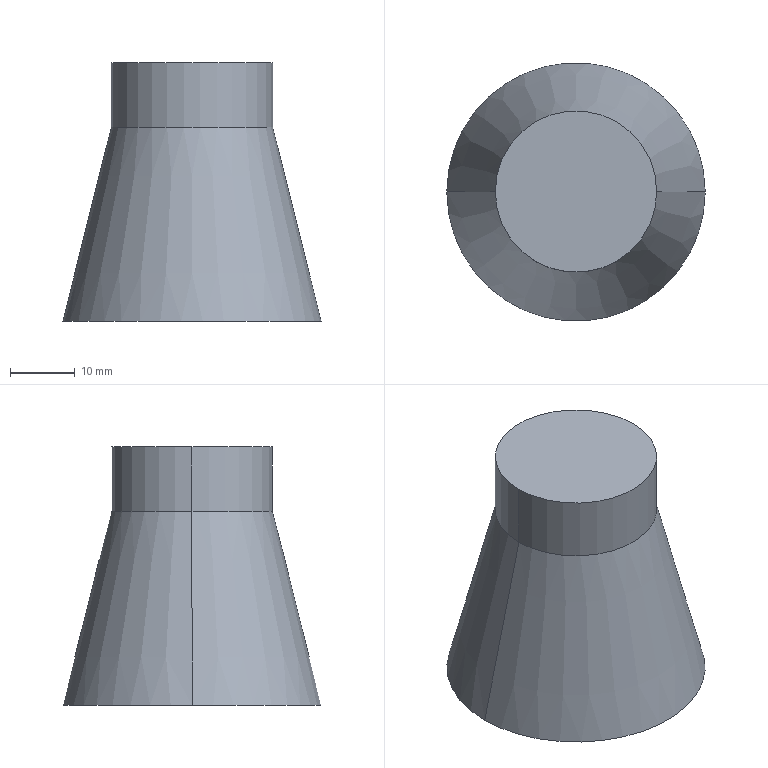Part | SolidWorks | features Blend 1, ICE 1 | 1 solid | 6 faces | box 40 x 40 x 40 mm | volume 30238 mm3 | cylinder 2 | cone 2 | plane 2 | commonest cylinder face diameters 25 x2
STEP:
#1=CARTESIAN_POINT('',(12.5,0.,40.));
#2=VERTEX_POINT('',#1);
#3=CARTESIAN_POINT('',(-12.5,0.,40.));
#4=VERTEX_POINT('',#3);
#5=CARTESIAN_POINT('',(0.,0.,40.));
#6=DIRECTION('',(0.,0.,1.));
#7=DIRECTION('',(1.,0.,0.));
#8=AXIS2_PLACEMENT_3D('',#5,#6,#7);
#9=CIRCLE('',#8,12.5);
#10=EDGE_CURVE('',#2,#4,#9,.T.);
#11=ORIENTED_EDGE('',*,*,#10,.F.);
#12=CARTESIAN_POINT('',(12.5,0.,30.));
#13=VERTEX_POINT('',#12);
#14=CARTESIAN_POINT('',(12.5,0.,40.));
#15=DIRECTION('',(0.,0.,-1.));
#16=VECTOR('',#15,1000.);
#17=LINE('',#14,#16);
#18=EDGE_CURVE('',#2,#13,#17,.T.);
#19=ORIENTED_EDGE('',*,*,#18,.T.);
#20=CARTESIAN_POINT('',(-12.5,0.,30.));
#21=VERTEX_POINT('',#20);
#22=CARTESIAN_POINT('',(0.,0.,30.));
#23=DIRECTION('',(0.,0.,1.));
#24=DIRECTION('',(1.,0.,0.));
#25=AXIS2_PLACEMENT_3D('',#22,#23,#24);
#26=CIRCLE('',#25,12.5);
#27=EDGE_CURVE('',#13,#21,#26,.T.);
#28=ORIENTED_EDGE('',*,*,#27,.T.);
#29=CARTESIAN_POINT('',(-12.5,0.,40.));
#30=DIRECTION('',(0.,0.,-1.));
#31=VECTOR('',#30,1000.);
#32=LINE('',#29,#31);
#33=EDGE_CURVE('',#4,#21,#32,.T.);
#34=ORIENTED_EDGE('',*,*,#33,.F.);
#35=EDGE_LOOP('',(#11,#19,#28,#34));
#36=FACE_OUTER_BOUND('',#35,.T.);
#37=CARTESIAN_POINT('',(0.,0.,40.));
#38=DIRECTION('',(0.,0.,-1.));
#39=DIRECTION('',(-1.,0.,0.));
#40=AXIS2_PLACEMENT_3D('',#37,#38,#39);
#41=CYLINDRICAL_SURFACE('',#40,12.5);
#42=ADVANCED_FACE('',(#36),#41,.T.);
#43=ORIENTED_EDGE('',*,*,#27,.F.);
#44=CARTESIAN_POINT('',(20.,0.,0.));
#45=VERTEX_POINT('',#44);
#46=CARTESIAN_POINT('',(12.5,0.,30.));
#47=DIRECTION('',(0.2425,0.,-0.9701));
#48=VECTOR('',#47,1000.);
#49=LINE('',#46,#48);
#50=EDGE_CURVE('',#13,#45,#49,.T.);
#51=ORIENTED_EDGE('',*,*,#50,.T.);
#52=CARTESIAN_POINT('',(-20.,0.,0.));
#53=VERTEX_POINT('',#52);
#54=CARTESIAN_POINT('',(0.,0.,0.));
#55=DIRECTION('',(0.,0.,1.));
#56=DIRECTION('',(1.,0.,0.));
#57=AXIS2_PLACEMENT_3D('',#54,#55,#56);
#58=CIRCLE('',#57,20.);
#59=EDGE_CURVE('',#45,#53,#58,.T.);
#60=ORIENTED_EDGE('',*,*,#59,.T.);
#61=CARTESIAN_POINT('',(-12.5,0.,30.));
#62=DIRECTION('',(-0.2425,0.,-0.9701));
#63=VECTOR('',#62,1000.);
#64=LINE('',#61,#63);
#65=EDGE_CURVE('',#21,#53,#64,.T.);
#66=ORIENTED_EDGE('',*,*,#65,.F.);
#67=EDGE_LOOP('',(#43,#51,#60,#66));
#68=FACE_OUTER_BOUND('',#67,.T.);
#69=CARTESIAN_POINT('',(0.,0.,30.));
#70=DIRECTION('',(0.,0.,-1.));
#71=DIRECTION('',(-1.,0.,0.));
#72=AXIS2_PLACEMENT_3D('',#69,#70,#71);
#73=CONICAL_SURFACE('',#72,12.5,0.245);
#74=ADVANCED_FACE('',(#68),#73,.T.);
#75=CARTESIAN_POINT('',(0.,0.,0.));
#76=DIRECTION('',(0.,0.,1.));
#77=DIRECTION('',(1.,0.,0.));
#78=AXIS2_PLACEMENT_3D('',#75,#76,#77);
#79=CIRCLE('',#78,20.);
#80=EDGE_CURVE('',#53,#45,#79,.T.);
#81=ORIENTED_EDGE('',*,*,#80,.F.);
#82=ORIENTED_EDGE('',*,*,#59,.F.);
#83=EDGE_LOOP('',(#81,#82));
#84=FACE_OUTER_BOUND('',#83,.T.);
#85=CARTESIAN_POINT('',(0.,0.,0.));
#86=DIRECTION('',(0.,0.,1.));
#87=DIRECTION('',(1.,0.,0.));
#88=AXIS2_PLACEMENT_3D('',#85,#86,#87);
#89=PLANE('',#88);
#90=ADVANCED_FACE('',(#84),#89,.F.);
#91=ORIENTED_EDGE('',*,*,#50,.F.);
#92=CARTESIAN_POINT('',(0.,0.,30.));
#93=DIRECTION('',(0.,0.,1.));
#94=DIRECTION('',(1.,0.,0.));
#95=AXIS2_PLACEMENT_3D('',#92,#93,#94);
#96=CIRCLE('',#95,12.5);
#97=EDGE_CURVE('',#21,#13,#96,.T.);
#98=ORIENTED_EDGE('',*,*,#97,.F.);
#99=ORIENTED_EDGE('',*,*,#65,.T.);
#100=ORIENTED_EDGE('',*,*,#80,.T.);
#101=EDGE_LOOP('',(#91,#98,#99,#100));
#102=FACE_OUTER_BOUND('',#101,.T.);
#103=CARTESIAN_POINT('',(0.,0.,30.));
#104=DIRECTION('',(0.,0.,-1.));
#105=DIRECTION('',(-1.,0.,0.));
#106=AXIS2_PLACEMENT_3D('',#103,#104,#105);
#107=CONICAL_SURFACE('',#106,12.5,0.245);
#108=ADVANCED_FACE('',(#102),#107,.T.);
#109=ORIENTED_EDGE('',*,*,#18,.F.);
#110=CARTESIAN_POINT('',(0.,0.,40.));
#111=DIRECTION('',(0.,0.,1.));
#112=DIRECTION('',(1.,0.,0.));
#113=AXIS2_PLACEMENT_3D('',#110,#111,#112);
#114=CIRCLE('',#113,12.5);
#115=EDGE_CURVE('',#4,#2,#114,.T.);
#116=ORIENTED_EDGE('',*,*,#115,.F.);
#117=ORIENTED_EDGE('',*,*,#33,.T.);
#118=ORIENTED_EDGE('',*,*,#97,.T.);
#119=EDGE_LOOP('',(#109,#116,#117,#118));
#120=FACE_OUTER_BOUND('',#119,.T.);
#121=CARTESIAN_POINT('',(0.,0.,40.));
#122=DIRECTION('',(0.,0.,-1.));
#123=DIRECTION('',(-1.,0.,0.));
#124=AXIS2_PLACEMENT_3D('',#121,#122,#123);
#125=CYLINDRICAL_SURFACE('',#124,12.5);
#126=ADVANCED_FACE('',(#120),#125,.T.);
#127=ORIENTED_EDGE('',*,*,#115,.T.);
#128=ORIENTED_EDGE('',*,*,#10,.T.);
#129=EDGE_LOOP('',(#127,#128));
#130=FACE_OUTER_BOUND('',#129,.T.);
#131=CARTESIAN_POINT('',(0.,0.,40.));
#132=DIRECTION('',(0.,0.,1.));
#133=DIRECTION('',(1.,0.,0.));
#134=AXIS2_PLACEMENT_3D('',#131,#132,#133);
#135=PLANE('',#134);
#136=ADVANCED_FACE('',(#130),#135,.T.);
#137=CLOSED_SHELL('',(#42,#74,#90,#108,#126,#136));
#138=MANIFOLD_SOLID_BREP('',#137);
#139=CARTESIAN_POINT('',(0.,0.,0.));
#140=DIRECTION('',(0.,0.,1.));
#141=DIRECTION('',(1.,0.,0.));
#142=AXIS2_PLACEMENT_3D('',#139,#140,#141);
#143=(LENGTH_UNIT()NAMED_UNIT(*)SI_UNIT(.MILLI.,.METRE.));
#144=UNCERTAINTY_MEASURE_WITH_UNIT(LENGTH_MEASURE(0.00001),#143,'','');
#145=(NAMED_UNIT(*)PLANE_ANGLE_UNIT()SI_UNIT($,.RADIAN.));
#146=(NAMED_UNIT(*)SI_UNIT($,.STERADIAN.)SOLID_ANGLE_UNIT());
#147=(GEOMETRIC_REPRESENTATION_CONTEXT(3)GLOBAL_UNCERTAINTY_ASSIGNED_CONTEXT((#144))GLOBAL_UNIT_ASSIGNED_CONTEXT((#143,#145,#146))REPRESENTATION_CONTEXT('',''));
#148=ADVANCED_BREP_SHAPE_REPRESENTATION('',(#138,#142),#147);